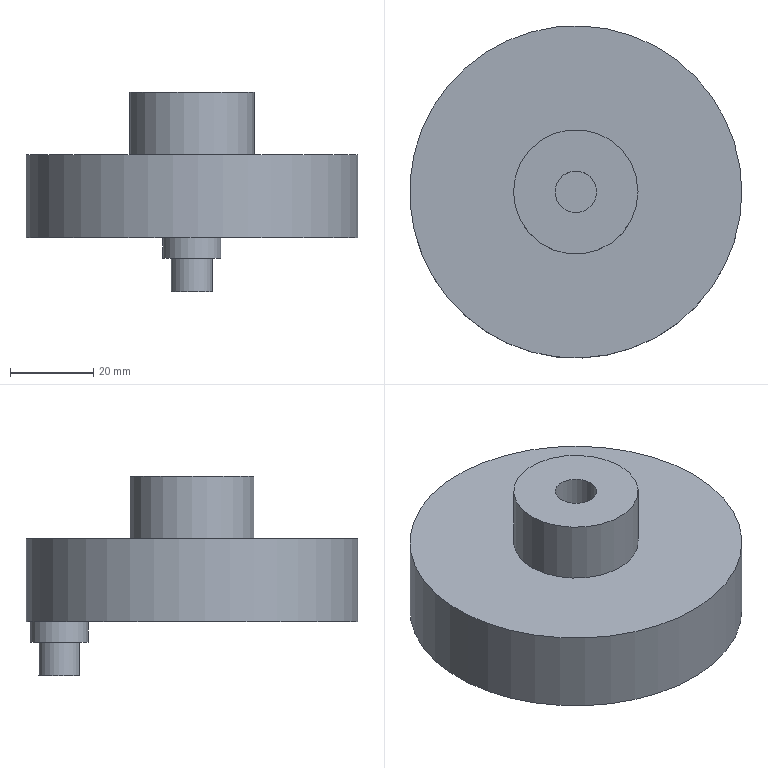Part | STEP file | tieqianqubin | 1 solid | 11 faces | box 80 x 80 x 48 mm | volume 111746 mm3 | plane 6 | cylinder 5 | commonest cylinder face diameters 10 x2 14 x1 30 x1 80 x1
STEP:
#1=CARTESIAN_POINT('',(0.,0.,0.));
#2=DIRECTION('',(0.,0.,1.));
#3=DIRECTION('',(1.,0.,0.));
#4=AXIS2_PLACEMENT_3D('',#1,#2,#3);
#5=CARTESIAN_POINT('',(-7.,32.,-5.));
#6=VERTEX_POINT('',#5);
#7=CARTESIAN_POINT('',(7.,32.,-5.));
#8=VERTEX_POINT('',#7);
#9=CARTESIAN_POINT('',(0.,32.,-5.));
#10=DIRECTION('',(0.,0.,-1.));
#11=DIRECTION('',(-1.,0.,0.));
#12=AXIS2_PLACEMENT_3D('',#9,#10,#11);
#13=CIRCLE('',#12,7.);
#14=CARTESIAN_POINT('',(0.,0.,-5.));
#15=DIRECTION('',(0.,0.,-1.));
#16=DIRECTION('',(-1.,0.,0.));
#17=AXIS2_PLACEMENT_3D('',#14,#15,#16);
#18=PLANE('',#17);
#19=CARTESIAN_POINT('',(0.,32.));
#20=DIRECTION('',(1.,0.));
#21=AXIS2_PLACEMENT_2D('',#19,#20);
#22=CIRCLE('',#21,7.);
#23=(GEOMETRIC_REPRESENTATION_CONTEXT(2)PARAMETRIC_REPRESENTATION_CONTEXT()REPRESENTATION_CONTEXT('',''));
#24=DEFINITIONAL_REPRESENTATION('',(#22),#23);
#25=PCURVE('',#18,#24);
#26=CARTESIAN_POINT('',(0.,32.,-5.));
#27=DIRECTION('',(0.,0.,1.));
#28=DIRECTION('',(1.,0.,0.));
#29=AXIS2_PLACEMENT_3D('',#26,#27,#28);
#30=CYLINDRICAL_SURFACE('',#29,7.);
#31=CARTESIAN_POINT('',(3.142,0.));
#32=DIRECTION('',(-1.,0.));
#33=VECTOR('',#32,1.);
#34=LINE('',#31,#33);
#35=(GEOMETRIC_REPRESENTATION_CONTEXT(2)PARAMETRIC_REPRESENTATION_CONTEXT()REPRESENTATION_CONTEXT('',''));
#36=DEFINITIONAL_REPRESENTATION('',(#34),#35);
#37=PCURVE('',#30,#36);
#38=SURFACE_CURVE('',#13,(#25,#37),.PCURVE_S1.);
#39=EDGE_CURVE('',#6,#8,#38,.T.);
#40=ORIENTED_EDGE('',*,*,#39,.T.);
#41=CARTESIAN_POINT('',(0.,32.,-5.));
#42=DIRECTION('',(0.,0.,-1.));
#43=DIRECTION('',(-1.,0.,0.));
#44=AXIS2_PLACEMENT_3D('',#41,#42,#43);
#45=CIRCLE('',#44,7.);
#46=CARTESIAN_POINT('',(0.,32.));
#47=DIRECTION('',(1.,0.));
#48=AXIS2_PLACEMENT_2D('',#46,#47);
#49=CIRCLE('',#48,7.);
#50=(GEOMETRIC_REPRESENTATION_CONTEXT(2)PARAMETRIC_REPRESENTATION_CONTEXT()REPRESENTATION_CONTEXT('',''));
#51=DEFINITIONAL_REPRESENTATION('',(#49),#50);
#52=PCURVE('',#18,#51);
#53=CARTESIAN_POINT('',(9.425,0.));
#54=DIRECTION('',(-1.,0.));
#55=VECTOR('',#54,1.);
#56=LINE('',#53,#55);
#57=(GEOMETRIC_REPRESENTATION_CONTEXT(2)PARAMETRIC_REPRESENTATION_CONTEXT()REPRESENTATION_CONTEXT('',''));
#58=DEFINITIONAL_REPRESENTATION('',(#56),#57);
#59=PCURVE('',#30,#58);
#60=SURFACE_CURVE('',#45,(#52,#59),.PCURVE_S1.);
#61=EDGE_CURVE('',#8,#6,#60,.T.);
#62=ORIENTED_EDGE('',*,*,#61,.T.);
#63=EDGE_LOOP('',(#40,#62));
#64=FACE_BOUND('',#63,.T.);
#65=CARTESIAN_POINT('',(-5.,32.,-5.));
#66=VERTEX_POINT('',#65);
#67=CARTESIAN_POINT('',(0.,32.,-5.));
#68=DIRECTION('',(0.,0.,-1.));
#69=DIRECTION('',(-1.,0.,0.));
#70=AXIS2_PLACEMENT_3D('',#67,#68,#69);
#71=CIRCLE('',#70,5.);
#72=CARTESIAN_POINT('',(0.,32.));
#73=DIRECTION('',(1.,0.));
#74=AXIS2_PLACEMENT_2D('',#72,#73);
#75=CIRCLE('',#74,5.);
#76=(GEOMETRIC_REPRESENTATION_CONTEXT(2)PARAMETRIC_REPRESENTATION_CONTEXT()REPRESENTATION_CONTEXT('',''));
#77=DEFINITIONAL_REPRESENTATION('',(#75),#76);
#78=PCURVE('',#18,#77);
#79=CARTESIAN_POINT('',(0.,32.,-13.));
#80=DIRECTION('',(0.,0.,1.));
#81=DIRECTION('',(1.,0.,0.));
#82=AXIS2_PLACEMENT_3D('',#79,#80,#81);
#83=CYLINDRICAL_SURFACE('',#82,5.);
#84=CARTESIAN_POINT('',(9.425,8.));
#85=DIRECTION('',(-1.,0.));
#86=VECTOR('',#85,1.);
#87=LINE('',#84,#86);
#88=(GEOMETRIC_REPRESENTATION_CONTEXT(2)PARAMETRIC_REPRESENTATION_CONTEXT()REPRESENTATION_CONTEXT('',''));
#89=DEFINITIONAL_REPRESENTATION('',(#87),#88);
#90=PCURVE('',#83,#89);
#91=SURFACE_CURVE('',#71,(#78,#90),.PCURVE_S1.);
#92=EDGE_CURVE('',#66,#66,#91,.T.);
#93=ORIENTED_EDGE('',*,*,#92,.F.);
#94=EDGE_LOOP('',(#93));
#95=FACE_BOUND('',#94,.T.);
#96=ADVANCED_FACE('',(#64,#95),#18,.T.);
#97=CARTESIAN_POINT('',(40.,0.,0.));
#98=VERTEX_POINT('',#97);
#99=CARTESIAN_POINT('',(0.,0.,0.));
#100=DIRECTION('',(0.,0.,1.));
#101=DIRECTION('',(1.,0.,0.));
#102=AXIS2_PLACEMENT_3D('',#99,#100,#101);
#103=CIRCLE('',#102,40.);
#104=CARTESIAN_POINT('',(0.,0.,0.));
#105=DIRECTION('',(0.,0.,1.));
#106=DIRECTION('',(1.,0.,0.));
#107=AXIS2_PLACEMENT_3D('',#104,#105,#106);
#108=PLANE('',#107);
#109=CARTESIAN_POINT('',(0.,0.));
#110=DIRECTION('',(1.,0.));
#111=AXIS2_PLACEMENT_2D('',#109,#110);
#112=CIRCLE('',#111,40.);
#113=(GEOMETRIC_REPRESENTATION_CONTEXT(2)PARAMETRIC_REPRESENTATION_CONTEXT()REPRESENTATION_CONTEXT('',''));
#114=DEFINITIONAL_REPRESENTATION('',(#112),#113);
#115=PCURVE('',#108,#114);
#116=CARTESIAN_POINT('',(0.,0.,20.));
#117=DIRECTION('',(0.,0.,-1.));
#118=DIRECTION('',(-1.,0.,0.));
#119=AXIS2_PLACEMENT_3D('',#116,#117,#118);
#120=CYLINDRICAL_SURFACE('',#119,40.);
#121=CARTESIAN_POINT('',(9.425,20.));
#122=DIRECTION('',(-1.,0.));
#123=VECTOR('',#122,1.);
#124=LINE('',#121,#123);
#125=(GEOMETRIC_REPRESENTATION_CONTEXT(2)PARAMETRIC_REPRESENTATION_CONTEXT()REPRESENTATION_CONTEXT('',''));
#126=DEFINITIONAL_REPRESENTATION('',(#124),#125);
#127=PCURVE('',#120,#126);
#128=SURFACE_CURVE('',#103,(#115,#127),.PCURVE_S1.);
#129=EDGE_CURVE('',#98,#98,#128,.T.);
#130=ORIENTED_EDGE('',*,*,#129,.F.);
#131=EDGE_LOOP('',(#130));
#132=FACE_BOUND('',#131,.T.);
#133=CARTESIAN_POINT('',(7.,32.,0.));
#134=VERTEX_POINT('',#133);
#135=CARTESIAN_POINT('',(0.,32.,0.));
#136=DIRECTION('',(0.,0.,-1.));
#137=DIRECTION('',(1.,0.,0.));
#138=AXIS2_PLACEMENT_3D('',#135,#136,#137);
#139=CIRCLE('',#138,7.);
#140=CARTESIAN_POINT('',(7.,32.));
#141=CARTESIAN_POINT('',(7.,19.876));
#142=CARTESIAN_POINT('',(-3.5,25.938));
#143=CARTESIAN_POINT('',(-14.,32.));
#144=CARTESIAN_POINT('',(-3.5,38.062));
#145=CARTESIAN_POINT('',(7.,44.124));
#146=CARTESIAN_POINT('',(7.,32.));
#147=(BOUNDED_CURVE()B_SPLINE_CURVE(2,(#140,#141,#142,#143,#144,#145,#146),.UNSPECIFIED.,.T.,.F.)B_SPLINE_CURVE_WITH_KNOTS((1,2,2,2,2,1),(-2.094,0.,2.094,4.189,6.283,8.378),.UNSPECIFIED.)CURVE()GEOMETRIC_REPRESENTATION_ITEM()RATIONAL_B_SPLINE_CURVE((1.,0.5,1.,0.5,1.,0.5,1.))REPRESENTATION_ITEM(''));
#148=(GEOMETRIC_REPRESENTATION_CONTEXT(2)PARAMETRIC_REPRESENTATION_CONTEXT()REPRESENTATION_CONTEXT('',''));
#149=DEFINITIONAL_REPRESENTATION('',(#147),#148);
#150=PCURVE('',#108,#149);
#151=CARTESIAN_POINT('',(6.283,5.));
#152=DIRECTION('',(-1.,0.));
#153=VECTOR('',#152,1.);
#154=LINE('',#151,#153);
#155=(GEOMETRIC_REPRESENTATION_CONTEXT(2)PARAMETRIC_REPRESENTATION_CONTEXT()REPRESENTATION_CONTEXT('',''));
#156=DEFINITIONAL_REPRESENTATION('',(#154),#155);
#157=PCURVE('',#30,#156);
#158=SURFACE_CURVE('',#139,(#150,#157),.PCURVE_S1.);
#159=EDGE_CURVE('',#134,#134,#158,.T.);
#160=ORIENTED_EDGE('',*,*,#159,.F.);
#161=EDGE_LOOP('',(#160));
#162=FACE_BOUND('',#161,.T.);
#163=ADVANCED_FACE('',(#132,#162),#108,.F.);
#164=CARTESIAN_POINT('',(40.,0.,20.));
#165=VERTEX_POINT('',#164);
#166=CARTESIAN_POINT('',(0.,0.,20.));
#167=DIRECTION('',(0.,0.,1.));
#168=DIRECTION('',(1.,0.,0.));
#169=AXIS2_PLACEMENT_3D('',#166,#167,#168);
#170=CIRCLE('',#169,40.);
#171=CARTESIAN_POINT('',(0.,0.,20.));
#172=DIRECTION('',(0.,0.,1.));
#173=DIRECTION('',(1.,0.,0.));
#174=AXIS2_PLACEMENT_3D('',#171,#172,#173);
#175=PLANE('',#174);
#176=CARTESIAN_POINT('',(0.,0.));
#177=DIRECTION('',(1.,0.));
#178=AXIS2_PLACEMENT_2D('',#176,#177);
#179=CIRCLE('',#178,40.);
#180=(GEOMETRIC_REPRESENTATION_CONTEXT(2)PARAMETRIC_REPRESENTATION_CONTEXT()REPRESENTATION_CONTEXT('',''));
#181=DEFINITIONAL_REPRESENTATION('',(#179),#180);
#182=PCURVE('',#175,#181);
#183=CARTESIAN_POINT('',(9.425,0.));
#184=DIRECTION('',(-1.,0.));
#185=VECTOR('',#184,1.);
#186=LINE('',#183,#185);
#187=(GEOMETRIC_REPRESENTATION_CONTEXT(2)PARAMETRIC_REPRESENTATION_CONTEXT()REPRESENTATION_CONTEXT('',''));
#188=DEFINITIONAL_REPRESENTATION('',(#186),#187);
#189=PCURVE('',#120,#188);
#190=SURFACE_CURVE('',#170,(#182,#189),.PCURVE_S1.);
#191=EDGE_CURVE('',#165,#165,#190,.T.);
#192=ORIENTED_EDGE('',*,*,#191,.T.);
#193=EDGE_LOOP('',(#192));
#194=FACE_BOUND('',#193,.T.);
#195=CARTESIAN_POINT('',(15.,0.,20.));
#196=VERTEX_POINT('',#195);
#197=CARTESIAN_POINT('',(0.,0.,20.));
#198=DIRECTION('',(0.,0.,1.));
#199=DIRECTION('',(1.,0.,0.));
#200=AXIS2_PLACEMENT_3D('',#197,#198,#199);
#201=CIRCLE('',#200,15.);
#202=CARTESIAN_POINT('',(0.,0.));
#203=DIRECTION('',(1.,0.));
#204=AXIS2_PLACEMENT_2D('',#202,#203);
#205=CIRCLE('',#204,15.);
#206=(GEOMETRIC_REPRESENTATION_CONTEXT(2)PARAMETRIC_REPRESENTATION_CONTEXT()REPRESENTATION_CONTEXT('',''));
#207=DEFINITIONAL_REPRESENTATION('',(#205),#206);
#208=PCURVE('',#175,#207);
#209=CARTESIAN_POINT('',(0.,0.,35.));
#210=DIRECTION('',(0.,0.,-1.));
#211=DIRECTION('',(-1.,0.,0.));
#212=AXIS2_PLACEMENT_3D('',#209,#210,#211);
#213=CYLINDRICAL_SURFACE('',#212,15.);
#214=CARTESIAN_POINT('',(9.425,15.));
#215=DIRECTION('',(-1.,0.));
#216=VECTOR('',#215,1.);
#217=LINE('',#214,#216);
#218=(GEOMETRIC_REPRESENTATION_CONTEXT(2)PARAMETRIC_REPRESENTATION_CONTEXT()REPRESENTATION_CONTEXT('',''));
#219=DEFINITIONAL_REPRESENTATION('',(#217),#218);
#220=PCURVE('',#213,#219);
#221=SURFACE_CURVE('',#201,(#208,#220),.PCURVE_S1.);
#222=EDGE_CURVE('',#196,#196,#221,.T.);
#223=ORIENTED_EDGE('',*,*,#222,.F.);
#224=EDGE_LOOP('',(#223));
#225=FACE_BOUND('',#224,.T.);
#226=ADVANCED_FACE('',(#194,#225),#175,.T.);
#227=ORIENTED_EDGE('',*,*,#191,.F.);
#228=CARTESIAN_POINT('',(40.,0.,20.));
#229=CARTESIAN_POINT('',(40.,0.,0.));
#230=B_SPLINE_CURVE_WITH_KNOTS('',1,(#228,#229),.UNSPECIFIED.,.F.,.F.,(2,2),(0.,20.),.PIECEWISE_BEZIER_KNOTS.);
#231=CARTESIAN_POINT('',(9.425,0.));
#232=DIRECTION('',(0.,1.));
#233=VECTOR('',#232,1.);
#234=LINE('',#231,#233);
#235=(GEOMETRIC_REPRESENTATION_CONTEXT(2)PARAMETRIC_REPRESENTATION_CONTEXT()REPRESENTATION_CONTEXT('',''));
#236=DEFINITIONAL_REPRESENTATION('',(#234),#235);
#237=PCURVE('',#120,#236);
#238=CARTESIAN_POINT('',(3.142,0.));
#239=DIRECTION('',(0.,1.));
#240=VECTOR('',#239,1.);
#241=LINE('',#238,#240);
#242=(GEOMETRIC_REPRESENTATION_CONTEXT(2)PARAMETRIC_REPRESENTATION_CONTEXT()REPRESENTATION_CONTEXT('',''));
#243=DEFINITIONAL_REPRESENTATION('',(#241),#242);
#244=PCURVE('',#120,#243);
#245=SEAM_CURVE('',#230,(#237,#244),.PCURVE_S1.);
#246=EDGE_CURVE('',#165,#98,#245,.T.);
#247=ORIENTED_EDGE('',*,*,#246,.T.);
#248=ORIENTED_EDGE('',*,*,#129,.T.);
#249=ORIENTED_EDGE('',*,*,#246,.F.);
#250=EDGE_LOOP('',(#227,#247,#248,#249));
#251=FACE_BOUND('',#250,.T.);
#252=ADVANCED_FACE('',(#251),#120,.T.);
#253=CARTESIAN_POINT('',(15.,0.,35.));
#254=VERTEX_POINT('',#253);
#255=CARTESIAN_POINT('',(0.,0.,35.));
#256=DIRECTION('',(0.,0.,1.));
#257=DIRECTION('',(1.,0.,0.));
#258=AXIS2_PLACEMENT_3D('',#255,#256,#257);
#259=CIRCLE('',#258,15.);
#260=CARTESIAN_POINT('',(9.425,0.));
#261=DIRECTION('',(-1.,0.));
#262=VECTOR('',#261,1.);
#263=LINE('',#260,#262);
#264=(GEOMETRIC_REPRESENTATION_CONTEXT(2)PARAMETRIC_REPRESENTATION_CONTEXT()REPRESENTATION_CONTEXT('',''));
#265=DEFINITIONAL_REPRESENTATION('',(#263),#264);
#266=PCURVE('',#213,#265);
#267=CARTESIAN_POINT('',(0.,0.,35.));
#268=DIRECTION('',(0.,0.,1.));
#269=DIRECTION('',(1.,0.,0.));
#270=AXIS2_PLACEMENT_3D('',#267,#268,#269);
#271=PLANE('',#270);
#272=CARTESIAN_POINT('',(0.,0.));
#273=DIRECTION('',(1.,0.));
#274=AXIS2_PLACEMENT_2D('',#272,#273);
#275=CIRCLE('',#274,15.);
#276=(GEOMETRIC_REPRESENTATION_CONTEXT(2)PARAMETRIC_REPRESENTATION_CONTEXT()REPRESENTATION_CONTEXT('',''));
#277=DEFINITIONAL_REPRESENTATION('',(#275),#276);
#278=PCURVE('',#271,#277);
#279=SURFACE_CURVE('',#259,(#266,#278),.PCURVE_S1.);
#280=EDGE_CURVE('',#254,#254,#279,.T.);
#281=ORIENTED_EDGE('',*,*,#280,.F.);
#282=CARTESIAN_POINT('',(15.,0.,35.));
#283=CARTESIAN_POINT('',(15.,0.,20.));
#284=B_SPLINE_CURVE_WITH_KNOTS('',1,(#282,#283),.UNSPECIFIED.,.F.,.F.,(2,2),(0.,15.),.PIECEWISE_BEZIER_KNOTS.);
#285=CARTESIAN_POINT('',(9.425,0.));
#286=DIRECTION('',(0.,1.));
#287=VECTOR('',#286,1.);
#288=LINE('',#285,#287);
#289=(GEOMETRIC_REPRESENTATION_CONTEXT(2)PARAMETRIC_REPRESENTATION_CONTEXT()REPRESENTATION_CONTEXT('',''));
#290=DEFINITIONAL_REPRESENTATION('',(#288),#289);
#291=PCURVE('',#213,#290);
#292=CARTESIAN_POINT('',(3.142,0.));
#293=DIRECTION('',(0.,1.));
#294=VECTOR('',#293,1.);
#295=LINE('',#292,#294);
#296=(GEOMETRIC_REPRESENTATION_CONTEXT(2)PARAMETRIC_REPRESENTATION_CONTEXT()REPRESENTATION_CONTEXT('',''));
#297=DEFINITIONAL_REPRESENTATION('',(#295),#296);
#298=PCURVE('',#213,#297);
#299=SEAM_CURVE('',#284,(#291,#298),.PCURVE_S1.);
#300=EDGE_CURVE('',#254,#196,#299,.T.);
#301=ORIENTED_EDGE('',*,*,#300,.T.);
#302=ORIENTED_EDGE('',*,*,#222,.T.);
#303=ORIENTED_EDGE('',*,*,#300,.F.);
#304=EDGE_LOOP('',(#281,#301,#302,#303));
#305=FACE_BOUND('',#304,.T.);
#306=ADVANCED_FACE('',(#305),#213,.T.);
#307=CARTESIAN_POINT('',(5.,0.,35.));
#308=VERTEX_POINT('',#307);
#309=CARTESIAN_POINT('',(0.,0.,35.));
#310=DIRECTION('',(0.,0.,1.));
#311=DIRECTION('',(1.,0.,0.));
#312=AXIS2_PLACEMENT_3D('',#309,#310,#311);
#313=CIRCLE('',#312,5.);
#314=CARTESIAN_POINT('',(0.,0.));
#315=DIRECTION('',(1.,0.));
#316=AXIS2_PLACEMENT_2D('',#314,#315);
#317=CIRCLE('',#316,5.);
#318=(GEOMETRIC_REPRESENTATION_CONTEXT(2)PARAMETRIC_REPRESENTATION_CONTEXT()REPRESENTATION_CONTEXT('',''));
#319=DEFINITIONAL_REPRESENTATION('',(#317),#318);
#320=PCURVE('',#271,#319);
#321=CARTESIAN_POINT('',(0.,0.,25.));
#322=DIRECTION('',(0.,0.,1.));
#323=DIRECTION('',(1.,0.,0.));
#324=AXIS2_PLACEMENT_3D('',#321,#322,#323);
#325=CYLINDRICAL_SURFACE('',#324,5.);
#326=CARTESIAN_POINT('',(0.,10.));
#327=DIRECTION('',(1.,0.));
#328=VECTOR('',#327,1.);
#329=LINE('',#326,#328);
#330=(GEOMETRIC_REPRESENTATION_CONTEXT(2)PARAMETRIC_REPRESENTATION_CONTEXT()REPRESENTATION_CONTEXT('',''));
#331=DEFINITIONAL_REPRESENTATION('',(#329),#330);
#332=PCURVE('',#325,#331);
#333=SURFACE_CURVE('',#313,(#320,#332),.PCURVE_S1.);
#334=EDGE_CURVE('',#308,#308,#333,.T.);
#335=ORIENTED_EDGE('',*,*,#334,.F.);
#336=EDGE_LOOP('',(#335));
#337=FACE_BOUND('',#336,.T.);
#338=ORIENTED_EDGE('',*,*,#280,.T.);
#339=EDGE_LOOP('',(#338));
#340=FACE_BOUND('',#339,.T.);
#341=ADVANCED_FACE('',(#337,#340),#271,.T.);
#342=ORIENTED_EDGE('',*,*,#61,.F.);
#343=CARTESIAN_POINT('',(7.,32.,-5.));
#344=CARTESIAN_POINT('',(7.,32.,0.));
#345=B_SPLINE_CURVE_WITH_KNOTS('',1,(#343,#344),.UNSPECIFIED.,.F.,.F.,(2,2),(0.,5.),.PIECEWISE_BEZIER_KNOTS.);
#346=CARTESIAN_POINT('',(6.283,0.));
#347=DIRECTION('',(0.,1.));
#348=VECTOR('',#347,1.);
#349=LINE('',#346,#348);
#350=(GEOMETRIC_REPRESENTATION_CONTEXT(2)PARAMETRIC_REPRESENTATION_CONTEXT()REPRESENTATION_CONTEXT('',''));
#351=DEFINITIONAL_REPRESENTATION('',(#349),#350);
#352=PCURVE('',#30,#351);
#353=CARTESIAN_POINT('',(0.,0.));
#354=DIRECTION('',(0.,1.));
#355=VECTOR('',#354,1.);
#356=LINE('',#353,#355);
#357=(GEOMETRIC_REPRESENTATION_CONTEXT(2)PARAMETRIC_REPRESENTATION_CONTEXT()REPRESENTATION_CONTEXT('',''));
#358=DEFINITIONAL_REPRESENTATION('',(#356),#357);
#359=PCURVE('',#30,#358);
#360=SEAM_CURVE('',#345,(#352,#359),.PCURVE_S1.);
#361=EDGE_CURVE('',#8,#134,#360,.T.);
#362=ORIENTED_EDGE('',*,*,#361,.T.);
#363=ORIENTED_EDGE('',*,*,#159,.T.);
#364=ORIENTED_EDGE('',*,*,#361,.F.);
#365=ORIENTED_EDGE('',*,*,#39,.F.);
#366=EDGE_LOOP('',(#342,#362,#363,#364,#365));
#367=FACE_BOUND('',#366,.T.);
#368=ADVANCED_FACE('',(#367),#30,.T.);
#369=CARTESIAN_POINT('',(-5.,32.,-13.));
#370=VERTEX_POINT('',#369);
#371=CARTESIAN_POINT('',(0.,32.,-13.));
#372=DIRECTION('',(0.,0.,-1.));
#373=DIRECTION('',(-1.,0.,0.));
#374=AXIS2_PLACEMENT_3D('',#371,#372,#373);
#375=CIRCLE('',#374,5.);
#376=CARTESIAN_POINT('',(9.425,0.));
#377=DIRECTION('',(-1.,0.));
#378=VECTOR('',#377,1.);
#379=LINE('',#376,#378);
#380=(GEOMETRIC_REPRESENTATION_CONTEXT(2)PARAMETRIC_REPRESENTATION_CONTEXT()REPRESENTATION_CONTEXT('',''));
#381=DEFINITIONAL_REPRESENTATION('',(#379),#380);
#382=PCURVE('',#83,#381);
#383=CARTESIAN_POINT('',(0.,32.,-13.));
#384=DIRECTION('',(0.,0.,-1.));
#385=DIRECTION('',(-1.,0.,0.));
#386=AXIS2_PLACEMENT_3D('',#383,#384,#385);
#387=PLANE('',#386);
#388=CARTESIAN_POINT('',(0.,0.));
#389=DIRECTION('',(1.,0.));
#390=AXIS2_PLACEMENT_2D('',#388,#389);
#391=CIRCLE('',#390,5.);
#392=(GEOMETRIC_REPRESENTATION_CONTEXT(2)PARAMETRIC_REPRESENTATION_CONTEXT()REPRESENTATION_CONTEXT('',''));
#393=DEFINITIONAL_REPRESENTATION('',(#391),#392);
#394=PCURVE('',#387,#393);
#395=SURFACE_CURVE('',#375,(#382,#394),.PCURVE_S1.);
#396=EDGE_CURVE('',#370,#370,#395,.T.);
#397=ORIENTED_EDGE('',*,*,#396,.F.);
#398=CARTESIAN_POINT('',(-5.,32.,-13.));
#399=CARTESIAN_POINT('',(-5.,32.,-5.));
#400=B_SPLINE_CURVE_WITH_KNOTS('',1,(#398,#399),.UNSPECIFIED.,.F.,.F.,(2,2),(0.,8.),.PIECEWISE_BEZIER_KNOTS.);
#401=CARTESIAN_POINT('',(9.425,0.));
#402=DIRECTION('',(0.,1.));
#403=VECTOR('',#402,1.);
#404=LINE('',#401,#403);
#405=(GEOMETRIC_REPRESENTATION_CONTEXT(2)PARAMETRIC_REPRESENTATION_CONTEXT()REPRESENTATION_CONTEXT('',''));
#406=DEFINITIONAL_REPRESENTATION('',(#404),#405);
#407=PCURVE('',#83,#406);
#408=CARTESIAN_POINT('',(3.142,0.));
#409=DIRECTION('',(0.,1.));
#410=VECTOR('',#409,1.);
#411=LINE('',#408,#410);
#412=(GEOMETRIC_REPRESENTATION_CONTEXT(2)PARAMETRIC_REPRESENTATION_CONTEXT()REPRESENTATION_CONTEXT('',''));
#413=DEFINITIONAL_REPRESENTATION('',(#411),#412);
#414=PCURVE('',#83,#413);
#415=SEAM_CURVE('',#400,(#407,#414),.PCURVE_S1.);
#416=EDGE_CURVE('',#370,#66,#415,.T.);
#417=ORIENTED_EDGE('',*,*,#416,.T.);
#418=ORIENTED_EDGE('',*,*,#92,.T.);
#419=ORIENTED_EDGE('',*,*,#416,.F.);
#420=EDGE_LOOP('',(#397,#417,#418,#419));
#421=FACE_BOUND('',#420,.T.);
#422=ADVANCED_FACE('',(#421),#83,.T.);
#423=ORIENTED_EDGE('',*,*,#396,.T.);
#424=EDGE_LOOP('',(#423));
#425=FACE_BOUND('',#424,.T.);
#426=ADVANCED_FACE('',(#425),#387,.T.);
#427=CARTESIAN_POINT('',(5.,0.,25.));
#428=VERTEX_POINT('',#427);
#429=CARTESIAN_POINT('',(0.,0.,25.));
#430=DIRECTION('',(0.,0.,1.));
#431=DIRECTION('',(1.,0.,0.));
#432=AXIS2_PLACEMENT_3D('',#429,#430,#431);
#433=CIRCLE('',#432,5.);
#434=CARTESIAN_POINT('',(0.,0.));
#435=DIRECTION('',(1.,0.));
#436=VECTOR('',#435,1.);
#437=LINE('',#434,#436);
#438=(GEOMETRIC_REPRESENTATION_CONTEXT(2)PARAMETRIC_REPRESENTATION_CONTEXT()REPRESENTATION_CONTEXT('',''));
#439=DEFINITIONAL_REPRESENTATION('',(#437),#438);
#440=PCURVE('',#325,#439);
#441=CARTESIAN_POINT('',(0.,0.,25.));
#442=DIRECTION('',(0.,0.,1.));
#443=DIRECTION('',(1.,0.,0.));
#444=AXIS2_PLACEMENT_3D('',#441,#442,#443);
#445=PLANE('',#444);
#446=CARTESIAN_POINT('',(0.,0.));
#447=DIRECTION('',(1.,0.));
#448=AXIS2_PLACEMENT_2D('',#446,#447);
#449=CIRCLE('',#448,5.);
#450=(GEOMETRIC_REPRESENTATION_CONTEXT(2)PARAMETRIC_REPRESENTATION_CONTEXT()REPRESENTATION_CONTEXT('',''));
#451=DEFINITIONAL_REPRESENTATION('',(#449),#450);
#452=PCURVE('',#445,#451);
#453=SURFACE_CURVE('',#433,(#440,#452),.PCURVE_S1.);
#454=EDGE_CURVE('',#428,#428,#453,.T.);
#455=ORIENTED_EDGE('',*,*,#454,.T.);
#456=CARTESIAN_POINT('',(5.,0.,25.));
#457=CARTESIAN_POINT('',(5.,0.,35.));
#458=B_SPLINE_CURVE_WITH_KNOTS('',1,(#456,#457),.UNSPECIFIED.,.F.,.F.,(2,2),(0.,10.),.PIECEWISE_BEZIER_KNOTS.);
#459=CARTESIAN_POINT('',(6.283,0.));
#460=DIRECTION('',(0.,1.));
#461=VECTOR('',#460,1.);
#462=LINE('',#459,#461);
#463=(GEOMETRIC_REPRESENTATION_CONTEXT(2)PARAMETRIC_REPRESENTATION_CONTEXT()REPRESENTATION_CONTEXT('',''));
#464=DEFINITIONAL_REPRESENTATION('',(#462),#463);
#465=PCURVE('',#325,#464);
#466=CARTESIAN_POINT('',(0.,0.));
#467=DIRECTION('',(0.,1.));
#468=VECTOR('',#467,1.);
#469=LINE('',#466,#468);
#470=(GEOMETRIC_REPRESENTATION_CONTEXT(2)PARAMETRIC_REPRESENTATION_CONTEXT()REPRESENTATION_CONTEXT('',''));
#471=DEFINITIONAL_REPRESENTATION('',(#469),#470);
#472=PCURVE('',#325,#471);
#473=SEAM_CURVE('',#458,(#465,#472),.PCURVE_S1.);
#474=EDGE_CURVE('',#428,#308,#473,.T.);
#475=ORIENTED_EDGE('',*,*,#474,.T.);
#476=ORIENTED_EDGE('',*,*,#334,.F.);
#477=ORIENTED_EDGE('',*,*,#474,.F.);
#478=EDGE_LOOP('',(#455,#475,#476,#477));
#479=FACE_BOUND('',#478,.F.);
#480=ADVANCED_FACE('',(#479),#325,.F.);
#481=ORIENTED_EDGE('',*,*,#454,.T.);
#482=EDGE_LOOP('',(#481));
#483=FACE_BOUND('',#482,.T.);
#484=ADVANCED_FACE('',(#483),#445,.T.);
#485=CLOSED_SHELL('',(#96,#163,#226,#252,#306,#341,#368,#422,#426,#480,#484));
#486=MANIFOLD_SOLID_BREP('',#485);
#487=(LENGTH_UNIT()NAMED_UNIT(*)SI_UNIT(.MILLI.,.METRE.));
#488=UNCERTAINTY_MEASURE_WITH_UNIT(LENGTH_MEASURE(0.000005),#487,'','');
#489=(NAMED_UNIT(*)PLANE_ANGLE_UNIT()SI_UNIT($,.RADIAN.));
#490=(NAMED_UNIT(*)SI_UNIT($,.STERADIAN.)SOLID_ANGLE_UNIT());
#491=(GEOMETRIC_REPRESENTATION_CONTEXT(3)GLOBAL_UNCERTAINTY_ASSIGNED_CONTEXT((#488))GLOBAL_UNIT_ASSIGNED_CONTEXT((#487,#489,#490))REPRESENTATION_CONTEXT('',''));
#492=ADVANCED_BREP_SHAPE_REPRESENTATION('',(#4,#486),#491);